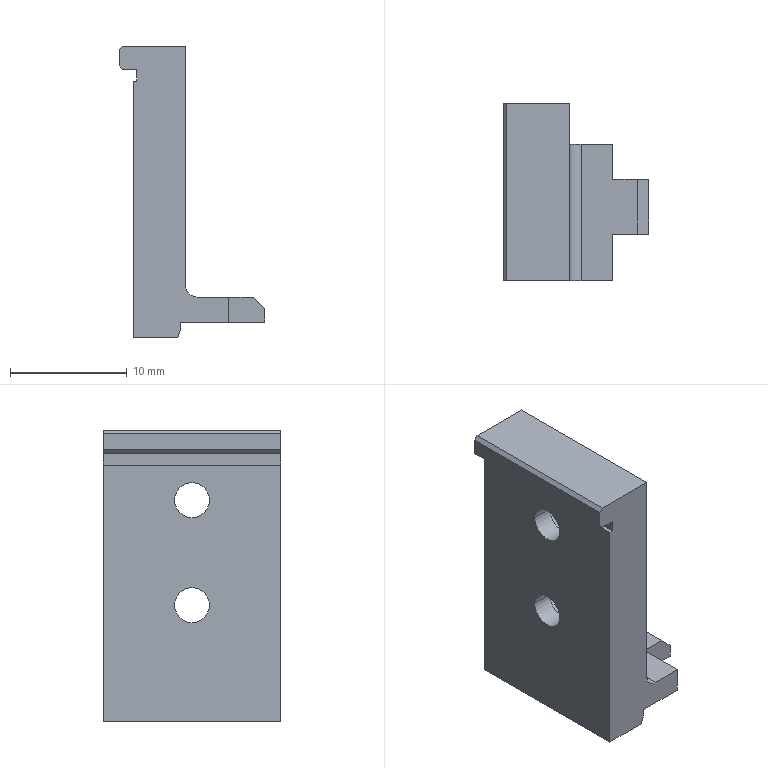Part | NX | 1 solid | 34 faces | box 12.5 x 15.2 x 25 mm | volume 1724 mm3 | plane 25 | cylinder 9 | commonest cylinder face diameters 3 x4 5 x4 2 x1
STEP:
#1=CARTESIAN_POINT('',(-1.77,0.,-1.43));
#2=VERTEX_POINT('',#1);
#3=CARTESIAN_POINT('',(-2.025,0.,-2.13));
#4=VERTEX_POINT('',#3);
#5=CARTESIAN_POINT('',(-1.25,0.,0.));
#6=DIRECTION('',(-0.342,0.,-0.9397));
#7=VECTOR('',#6,1000.);
#8=LINE('',#5,#7);
#9=EDGE_CURVE('',#2,#4,#8,.T.);
#10=ORIENTED_EDGE('',*,*,#9,.T.);
#11=CARTESIAN_POINT('',(-5.85,0.,-2.13));
#12=VERTEX_POINT('',#11);
#13=CARTESIAN_POINT('',(0.,0.,-2.13));
#14=DIRECTION('',(1.,0.,0.));
#15=VECTOR('',#14,1000.);
#16=LINE('',#13,#15);
#17=EDGE_CURVE('',#12,#4,#16,.T.);
#18=ORIENTED_EDGE('',*,*,#17,.F.);
#19=CARTESIAN_POINT('',(-5.85,0.,19.87));
#20=VERTEX_POINT('',#19);
#21=CARTESIAN_POINT('',(-5.85,0.,0.));
#22=DIRECTION('',(0.,0.,1.));
#23=VECTOR('',#22,1000.);
#24=LINE('',#21,#23);
#25=EDGE_CURVE('',#12,#20,#24,.T.);
#26=ORIENTED_EDGE('',*,*,#25,.T.);
#27=CARTESIAN_POINT('',(-5.55,0.,19.87));
#28=VERTEX_POINT('',#27);
#29=CARTESIAN_POINT('',(0.,0.,19.87));
#30=DIRECTION('',(1.,0.,0.));
#31=VECTOR('',#30,1000.);
#32=LINE('',#29,#31);
#33=EDGE_CURVE('',#20,#28,#32,.T.);
#34=ORIENTED_EDGE('',*,*,#33,.T.);
#35=CARTESIAN_POINT('',(-5.55,0.,20.87));
#36=VERTEX_POINT('',#35);
#37=CARTESIAN_POINT('',(-5.55,0.,0.));
#38=DIRECTION('',(0.,0.,1.));
#39=VECTOR('',#38,1000.);
#40=LINE('',#37,#39);
#41=EDGE_CURVE('',#28,#36,#40,.T.);
#42=ORIENTED_EDGE('',*,*,#41,.T.);
#43=CARTESIAN_POINT('',(-6.75,0.,20.87));
#44=VERTEX_POINT('',#43);
#45=CARTESIAN_POINT('',(0.,0.,20.87));
#46=DIRECTION('',(-1.,0.,0.));
#47=VECTOR('',#46,1000.);
#48=LINE('',#45,#47);
#49=EDGE_CURVE('',#36,#44,#48,.T.);
#50=ORIENTED_EDGE('',*,*,#49,.T.);
#51=CARTESIAN_POINT('',(-7.05,0.,21.17));
#52=VERTEX_POINT('',#51);
#53=CARTESIAN_POINT('',(14.12,0.,0.));
#54=DIRECTION('',(0.7071,0.,-0.7071));
#55=VECTOR('',#54,1000.);
#56=LINE('',#53,#55);
#57=EDGE_CURVE('',#52,#44,#56,.T.);
#58=ORIENTED_EDGE('',*,*,#57,.F.);
#59=CARTESIAN_POINT('',(-7.05,0.,22.57));
#60=VERTEX_POINT('',#59);
#61=CARTESIAN_POINT('',(-7.05,0.,0.));
#62=DIRECTION('',(0.,0.,1.));
#63=VECTOR('',#62,1000.);
#64=LINE('',#61,#63);
#65=EDGE_CURVE('',#52,#60,#64,.T.);
#66=ORIENTED_EDGE('',*,*,#65,.T.);
#67=CARTESIAN_POINT('',(-6.75,0.,22.87));
#68=VERTEX_POINT('',#67);
#69=CARTESIAN_POINT('',(-29.62,0.,0.));
#70=DIRECTION('',(0.7071,0.,0.7071));
#71=VECTOR('',#70,1000.);
#72=LINE('',#69,#71);
#73=EDGE_CURVE('',#60,#68,#72,.T.);
#74=ORIENTED_EDGE('',*,*,#73,.T.);
#75=CARTESIAN_POINT('',(-1.35,0.,22.87));
#76=VERTEX_POINT('',#75);
#77=CARTESIAN_POINT('',(0.,0.,22.87));
#78=DIRECTION('',(1.,0.,0.));
#79=VECTOR('',#78,1000.);
#80=LINE('',#77,#79);
#81=EDGE_CURVE('',#68,#76,#80,.T.);
#82=ORIENTED_EDGE('',*,*,#81,.T.);
#83=CARTESIAN_POINT('',(-1.35,0.,-0.78));
#84=VERTEX_POINT('',#83);
#85=CARTESIAN_POINT('',(-1.35,0.,0.));
#86=DIRECTION('',(0.,0.,1.));
#87=VECTOR('',#86,1000.);
#88=LINE('',#85,#87);
#89=EDGE_CURVE('',#84,#76,#88,.T.);
#90=ORIENTED_EDGE('',*,*,#89,.F.);
#91=CARTESIAN_POINT('',(-1.77,0.,-0.78));
#92=VERTEX_POINT('',#91);
#93=CARTESIAN_POINT('',(0.,0.,-0.78));
#94=DIRECTION('',(-1.,0.,0.));
#95=VECTOR('',#94,1000.);
#96=LINE('',#93,#95);
#97=EDGE_CURVE('',#84,#92,#96,.T.);
#98=ORIENTED_EDGE('',*,*,#97,.T.);
#99=CARTESIAN_POINT('',(-1.77,0.,0.));
#100=DIRECTION('',(0.,0.,-1.));
#101=VECTOR('',#100,1000.);
#102=LINE('',#99,#101);
#103=EDGE_CURVE('',#92,#2,#102,.T.);
#104=ORIENTED_EDGE('',*,*,#103,.T.);
#105=EDGE_LOOP('',(#10,#18,#26,#34,#42,#50,#58,#66,#74,#82,#90,#98,#104));
#106=FACE_BOUND('',#105,.T.);
#107=CARTESIAN_POINT('',(0.,0.,0.));
#108=DIRECTION('',(0.,-1.,0.));
#109=DIRECTION('',(0.,0.,-1.));
#110=AXIS2_PLACEMENT_3D('',#107,#108,#109);
#111=PLANE('',#110);
#112=ADVANCED_FACE('',(#106),#111,.F.);
#113=CARTESIAN_POINT('',(-1.77,-15.2,-1.43));
#114=VERTEX_POINT('',#113);
#115=CARTESIAN_POINT('',(-1.77,0.,-1.43));
#116=DIRECTION('',(0.,-1.,0.));
#117=VECTOR('',#116,1000.);
#118=LINE('',#115,#117);
#119=EDGE_CURVE('',#2,#114,#118,.T.);
#120=ORIENTED_EDGE('',*,*,#119,.F.);
#121=ORIENTED_EDGE('',*,*,#103,.F.);
#122=CARTESIAN_POINT('',(-1.77,-15.2,-0.78));
#123=VERTEX_POINT('',#122);
#124=CARTESIAN_POINT('',(-1.77,0.,-0.78));
#125=DIRECTION('',(0.,-1.,0.));
#126=VECTOR('',#125,1000.);
#127=LINE('',#124,#126);
#128=EDGE_CURVE('',#92,#123,#127,.T.);
#129=ORIENTED_EDGE('',*,*,#128,.T.);
#130=CARTESIAN_POINT('',(-1.77,-15.2,0.));
#131=DIRECTION('',(0.,0.,1.));
#132=VECTOR('',#131,1000.);
#133=LINE('',#130,#132);
#134=EDGE_CURVE('',#114,#123,#133,.T.);
#135=ORIENTED_EDGE('',*,*,#134,.F.);
#136=EDGE_LOOP('',(#120,#121,#129,#135));
#137=FACE_BOUND('',#136,.T.);
#138=CARTESIAN_POINT('',(-1.77,0.,-0.93));
#139=DIRECTION('',(1.,0.,0.));
#140=DIRECTION('',(0.,1.,0.));
#141=AXIS2_PLACEMENT_3D('',#138,#139,#140);
#142=PLANE('',#141);
#143=ADVANCED_FACE('',(#137),#142,.T.);
#144=CARTESIAN_POINT('',(-0.35,-15.2,1.37));
#145=VERTEX_POINT('',#144);
#146=CARTESIAN_POINT('',(2.35,-15.2,1.37));
#147=VERTEX_POINT('',#146);
#148=CARTESIAN_POINT('',(0.,-15.2,1.37));
#149=DIRECTION('',(1.,0.,0.));
#150=VECTOR('',#149,1000.);
#151=LINE('',#148,#150);
#152=EDGE_CURVE('',#145,#147,#151,.T.);
#153=ORIENTED_EDGE('',*,*,#152,.F.);
#154=CARTESIAN_POINT('',(-1.35,-15.2,2.37));
#155=VERTEX_POINT('',#154);
#156=CARTESIAN_POINT('',(-0.35,-15.2,2.37));
#157=DIRECTION('',(0.,1.,0.));
#158=DIRECTION('',(-1.,0.,0.));
#159=AXIS2_PLACEMENT_3D('',#156,#157,#158);
#160=CIRCLE('',#159,1.);
#161=EDGE_CURVE('',#145,#155,#160,.T.);
#162=ORIENTED_EDGE('',*,*,#161,.T.);
#163=CARTESIAN_POINT('',(-1.35,-15.2,22.87));
#164=VERTEX_POINT('',#163);
#165=CARTESIAN_POINT('',(-1.35,-15.2,0.));
#166=DIRECTION('',(0.,0.,-1.));
#167=VECTOR('',#166,1000.);
#168=LINE('',#165,#167);
#169=EDGE_CURVE('',#164,#155,#168,.T.);
#170=ORIENTED_EDGE('',*,*,#169,.F.);
#171=CARTESIAN_POINT('',(-6.75,-15.2,22.87));
#172=VERTEX_POINT('',#171);
#173=CARTESIAN_POINT('',(0.,-15.2,22.87));
#174=DIRECTION('',(-1.,0.,0.));
#175=VECTOR('',#174,1000.);
#176=LINE('',#173,#175);
#177=EDGE_CURVE('',#164,#172,#176,.T.);
#178=ORIENTED_EDGE('',*,*,#177,.T.);
#179=CARTESIAN_POINT('',(-7.05,-15.2,22.57));
#180=VERTEX_POINT('',#179);
#181=CARTESIAN_POINT('',(-29.62,-15.2,0.));
#182=DIRECTION('',(-0.7071,0.,-0.7071));
#183=VECTOR('',#182,1000.);
#184=LINE('',#181,#183);
#185=EDGE_CURVE('',#172,#180,#184,.T.);
#186=ORIENTED_EDGE('',*,*,#185,.T.);
#187=CARTESIAN_POINT('',(-7.05,-15.2,21.17));
#188=VERTEX_POINT('',#187);
#189=CARTESIAN_POINT('',(-7.05,-15.2,0.));
#190=DIRECTION('',(0.,0.,-1.));
#191=VECTOR('',#190,1000.);
#192=LINE('',#189,#191);
#193=EDGE_CURVE('',#180,#188,#192,.T.);
#194=ORIENTED_EDGE('',*,*,#193,.T.);
#195=CARTESIAN_POINT('',(-6.75,-15.2,20.87));
#196=VERTEX_POINT('',#195);
#197=CARTESIAN_POINT('',(14.12,-15.2,0.));
#198=DIRECTION('',(-0.7071,0.,0.7071));
#199=VECTOR('',#198,1000.);
#200=LINE('',#197,#199);
#201=EDGE_CURVE('',#196,#188,#200,.T.);
#202=ORIENTED_EDGE('',*,*,#201,.F.);
#203=CARTESIAN_POINT('',(-5.55,-15.2,20.87));
#204=VERTEX_POINT('',#203);
#205=CARTESIAN_POINT('',(0.,-15.2,20.87));
#206=DIRECTION('',(1.,0.,0.));
#207=VECTOR('',#206,1000.);
#208=LINE('',#205,#207);
#209=EDGE_CURVE('',#196,#204,#208,.T.);
#210=ORIENTED_EDGE('',*,*,#209,.T.);
#211=CARTESIAN_POINT('',(-5.55,-15.2,19.87));
#212=VERTEX_POINT('',#211);
#213=CARTESIAN_POINT('',(-5.55,-15.2,0.));
#214=DIRECTION('',(0.,0.,-1.));
#215=VECTOR('',#214,1000.);
#216=LINE('',#213,#215);
#217=EDGE_CURVE('',#204,#212,#216,.T.);
#218=ORIENTED_EDGE('',*,*,#217,.T.);
#219=CARTESIAN_POINT('',(-5.85,-15.2,19.87));
#220=VERTEX_POINT('',#219);
#221=CARTESIAN_POINT('',(0.,-15.2,19.87));
#222=DIRECTION('',(-1.,0.,0.));
#223=VECTOR('',#222,1000.);
#224=LINE('',#221,#223);
#225=EDGE_CURVE('',#212,#220,#224,.T.);
#226=ORIENTED_EDGE('',*,*,#225,.T.);
#227=CARTESIAN_POINT('',(-5.85,-15.2,-2.13));
#228=VERTEX_POINT('',#227);
#229=CARTESIAN_POINT('',(-5.85,-15.2,0.));
#230=DIRECTION('',(0.,0.,-1.));
#231=VECTOR('',#230,1000.);
#232=LINE('',#229,#231);
#233=EDGE_CURVE('',#220,#228,#232,.T.);
#234=ORIENTED_EDGE('',*,*,#233,.T.);
#235=CARTESIAN_POINT('',(-2.025,-15.2,-2.13));
#236=VERTEX_POINT('',#235);
#237=CARTESIAN_POINT('',(0.,-15.2,-2.13));
#238=DIRECTION('',(-1.,0.,0.));
#239=VECTOR('',#238,1000.);
#240=LINE('',#237,#239);
#241=EDGE_CURVE('',#236,#228,#240,.T.);
#242=ORIENTED_EDGE('',*,*,#241,.F.);
#243=CARTESIAN_POINT('',(-1.25,-15.2,0.));
#244=DIRECTION('',(0.342,0.,0.9397));
#245=VECTOR('',#244,1000.);
#246=LINE('',#243,#245);
#247=EDGE_CURVE('',#236,#114,#246,.T.);
#248=ORIENTED_EDGE('',*,*,#247,.T.);
#249=ORIENTED_EDGE('',*,*,#134,.T.);
#250=CARTESIAN_POINT('',(2.35,-15.2,-0.78));
#251=VERTEX_POINT('',#250);
#252=CARTESIAN_POINT('',(0.,-15.2,-0.78));
#253=DIRECTION('',(1.,0.,0.));
#254=VECTOR('',#253,1000.);
#255=LINE('',#252,#254);
#256=EDGE_CURVE('',#123,#251,#255,.T.);
#257=ORIENTED_EDGE('',*,*,#256,.T.);
#258=CARTESIAN_POINT('',(2.35,-15.2,0.));
#259=DIRECTION('',(0.,0.,-1.));
#260=VECTOR('',#259,1000.);
#261=LINE('',#258,#260);
#262=EDGE_CURVE('',#147,#251,#261,.T.);
#263=ORIENTED_EDGE('',*,*,#262,.F.);
#264=EDGE_LOOP('',(#153,#162,#170,#178,#186,#194,#202,#210,#218,#226,#234,#242,#248,#249,#257,#263));
#265=FACE_BOUND('',#264,.T.);
#266=CARTESIAN_POINT('',(-1.35,-15.2,0.));
#267=DIRECTION('',(0.,1.,0.));
#268=DIRECTION('',(1.,0.,0.));
#269=AXIS2_PLACEMENT_3D('',#266,#267,#268);
#270=PLANE('',#269);
#271=ADVANCED_FACE('',(#265),#270,.F.);
#272=CARTESIAN_POINT('',(-4.05,-5.1,7.87));
#273=VERTEX_POINT('',#272);
#274=CARTESIAN_POINT('',(-4.05,-10.1,7.87));
#275=VERTEX_POINT('',#274);
#276=CARTESIAN_POINT('',(-4.05,-7.6,7.87));
#277=DIRECTION('',(1.,0.,0.));
#278=DIRECTION('',(0.,-1.,0.));
#279=AXIS2_PLACEMENT_3D('',#276,#277,#278);
#280=CIRCLE('',#279,2.5);
#281=EDGE_CURVE('',#273,#275,#280,.T.);
#282=ORIENTED_EDGE('',*,*,#281,.T.);
#283=CARTESIAN_POINT('',(-4.05,-7.6,7.87));
#284=DIRECTION('',(1.,0.,0.));
#285=DIRECTION('',(0.,-1.,0.));
#286=AXIS2_PLACEMENT_3D('',#283,#284,#285);
#287=CIRCLE('',#286,2.5);
#288=EDGE_CURVE('',#275,#273,#287,.T.);
#289=ORIENTED_EDGE('',*,*,#288,.T.);
#290=EDGE_LOOP('',(#282,#289));
#291=FACE_BOUND('',#290,.T.);
#292=CARTESIAN_POINT('',(-4.05,-6.1,7.87));
#293=VERTEX_POINT('',#292);
#294=CARTESIAN_POINT('',(-4.05,-9.1,7.87));
#295=VERTEX_POINT('',#294);
#296=CARTESIAN_POINT('',(-4.05,-7.6,7.87));
#297=DIRECTION('',(1.,0.,0.));
#298=DIRECTION('',(0.,-1.,0.));
#299=AXIS2_PLACEMENT_3D('',#296,#297,#298);
#300=CIRCLE('',#299,1.5);
#301=EDGE_CURVE('',#293,#295,#300,.T.);
#302=ORIENTED_EDGE('',*,*,#301,.F.);
#303=CARTESIAN_POINT('',(-4.05,-7.6,7.87));
#304=DIRECTION('',(1.,0.,0.));
#305=DIRECTION('',(0.,-1.,0.));
#306=AXIS2_PLACEMENT_3D('',#303,#304,#305);
#307=CIRCLE('',#306,1.5);
#308=EDGE_CURVE('',#295,#293,#307,.T.);
#309=ORIENTED_EDGE('',*,*,#308,.F.);
#310=EDGE_LOOP('',(#302,#309));
#311=FACE_BOUND('',#310,.T.);
#312=CARTESIAN_POINT('',(-4.05,-7.6,7.87));
#313=DIRECTION('',(-1.,0.,0.));
#314=DIRECTION('',(0.,0.,1.));
#315=AXIS2_PLACEMENT_3D('',#312,#313,#314);
#316=PLANE('',#315);
#317=ADVANCED_FACE('',(#291,#311),#316,.F.);
#318=ORIENTED_EDGE('',*,*,#241,.T.);
#319=CARTESIAN_POINT('',(-5.85,0.,-2.13));
#320=DIRECTION('',(0.,1.,0.));
#321=VECTOR('',#320,1000.);
#322=LINE('',#319,#321);
#323=EDGE_CURVE('',#228,#12,#322,.T.);
#324=ORIENTED_EDGE('',*,*,#323,.T.);
#325=ORIENTED_EDGE('',*,*,#17,.T.);
#326=CARTESIAN_POINT('',(-2.025,0.,-2.13));
#327=DIRECTION('',(0.,-1.,0.));
#328=VECTOR('',#327,1000.);
#329=LINE('',#326,#328);
#330=EDGE_CURVE('',#4,#236,#329,.T.);
#331=ORIENTED_EDGE('',*,*,#330,.T.);
#332=EDGE_LOOP('',(#318,#324,#325,#331));
#333=FACE_BOUND('',#332,.T.);
#334=CARTESIAN_POINT('',(0.,0.,-2.13));
#335=DIRECTION('',(0.,0.,1.));
#336=DIRECTION('',(1.,0.,0.));
#337=AXIS2_PLACEMENT_3D('',#334,#335,#336);
#338=PLANE('',#337);
#339=ADVANCED_FACE('',(#333),#338,.F.);
#340=ORIENTED_EDGE('',*,*,#9,.F.);
#341=ORIENTED_EDGE('',*,*,#119,.T.);
#342=ORIENTED_EDGE('',*,*,#247,.F.);
#343=ORIENTED_EDGE('',*,*,#330,.F.);
#344=EDGE_LOOP('',(#340,#341,#342,#343));
#345=FACE_BOUND('',#344,.T.);
#346=CARTESIAN_POINT('',(-2.025,-15.2,-2.13));
#347=DIRECTION('',(0.9397,0.,-0.342));
#348=DIRECTION('',(0.,-1.,0.));
#349=AXIS2_PLACEMENT_3D('',#346,#347,#348);
#350=PLANE('',#349);
#351=ADVANCED_FACE('',(#345),#350,.T.);
#352=CARTESIAN_POINT('',(-5.85,0.,19.87));
#353=DIRECTION('',(0.,-1.,0.));
#354=VECTOR('',#353,1000.);
#355=LINE('',#352,#354);
#356=EDGE_CURVE('',#20,#220,#355,.T.);
#357=ORIENTED_EDGE('',*,*,#356,.T.);
#358=ORIENTED_EDGE('',*,*,#225,.F.);
#359=CARTESIAN_POINT('',(-5.55,0.,19.87));
#360=DIRECTION('',(0.,-1.,0.));
#361=VECTOR('',#360,1000.);
#362=LINE('',#359,#361);
#363=EDGE_CURVE('',#28,#212,#362,.T.);
#364=ORIENTED_EDGE('',*,*,#363,.F.);
#365=ORIENTED_EDGE('',*,*,#33,.F.);
#366=EDGE_LOOP('',(#357,#358,#364,#365));
#367=FACE_BOUND('',#366,.T.);
#368=CARTESIAN_POINT('',(-4.85,0.,19.87));
#369=DIRECTION('',(0.,0.,1.));
#370=DIRECTION('',(1.,0.,0.));
#371=AXIS2_PLACEMENT_3D('',#368,#369,#370);
#372=PLANE('',#371);
#373=ADVANCED_FACE('',(#367),#372,.T.);
#374=ORIENTED_EDGE('',*,*,#363,.T.);
#375=ORIENTED_EDGE('',*,*,#217,.F.);
#376=CARTESIAN_POINT('',(-5.55,0.,20.87));
#377=DIRECTION('',(0.,-1.,0.));
#378=VECTOR('',#377,1000.);
#379=LINE('',#376,#378);
#380=EDGE_CURVE('',#36,#204,#379,.T.);
#381=ORIENTED_EDGE('',*,*,#380,.F.);
#382=ORIENTED_EDGE('',*,*,#41,.F.);
#383=EDGE_LOOP('',(#374,#375,#381,#382));
#384=FACE_BOUND('',#383,.T.);
#385=CARTESIAN_POINT('',(-5.55,0.,19.87));
#386=DIRECTION('',(-1.,0.,0.));
#387=DIRECTION('',(0.,0.,1.));
#388=AXIS2_PLACEMENT_3D('',#385,#386,#387);
#389=PLANE('',#388);
#390=ADVANCED_FACE('',(#384),#389,.T.);
#391=CARTESIAN_POINT('',(-6.75,0.,20.87));
#392=DIRECTION('',(0.,1.,0.));
#393=VECTOR('',#392,1000.);
#394=LINE('',#391,#393);
#395=EDGE_CURVE('',#196,#44,#394,.T.);
#396=ORIENTED_EDGE('',*,*,#395,.T.);
#397=ORIENTED_EDGE('',*,*,#49,.F.);
#398=ORIENTED_EDGE('',*,*,#380,.T.);
#399=ORIENTED_EDGE('',*,*,#209,.F.);
#400=EDGE_LOOP('',(#396,#397,#398,#399));
#401=FACE_BOUND('',#400,.T.);
#402=CARTESIAN_POINT('',(-4.85,0.,20.87));
#403=DIRECTION('',(0.,0.,-1.));
#404=DIRECTION('',(0.,-1.,0.));
#405=AXIS2_PLACEMENT_3D('',#402,#403,#404);
#406=PLANE('',#405);
#407=ADVANCED_FACE('',(#401),#406,.T.);
#408=CARTESIAN_POINT('',(-7.05,0.,22.57));
#409=DIRECTION('',(0.,-1.,0.));
#410=VECTOR('',#409,1000.);
#411=LINE('',#408,#410);
#412=EDGE_CURVE('',#60,#180,#411,.T.);
#413=ORIENTED_EDGE('',*,*,#412,.F.);
#414=ORIENTED_EDGE('',*,*,#65,.F.);
#415=CARTESIAN_POINT('',(-7.05,0.,21.17));
#416=DIRECTION('',(0.,-1.,0.));
#417=VECTOR('',#416,1000.);
#418=LINE('',#415,#417);
#419=EDGE_CURVE('',#52,#188,#418,.T.);
#420=ORIENTED_EDGE('',*,*,#419,.T.);
#421=ORIENTED_EDGE('',*,*,#193,.F.);
#422=EDGE_LOOP('',(#413,#414,#420,#421));
#423=FACE_BOUND('',#422,.T.);
#424=CARTESIAN_POINT('',(-7.05,0.,20.87));
#425=DIRECTION('',(-1.,0.,0.));
#426=DIRECTION('',(0.,0.,1.));
#427=AXIS2_PLACEMENT_3D('',#424,#425,#426);
#428=PLANE('',#427);
#429=ADVANCED_FACE('',(#423),#428,.T.);
#430=CARTESIAN_POINT('',(-6.75,0.,22.87));
#431=DIRECTION('',(0.,1.,0.));
#432=VECTOR('',#431,1000.);
#433=LINE('',#430,#432);
#434=EDGE_CURVE('',#172,#68,#433,.T.);
#435=ORIENTED_EDGE('',*,*,#434,.F.);
#436=ORIENTED_EDGE('',*,*,#177,.F.);
#437=CARTESIAN_POINT('',(-1.35,0.,22.87));
#438=DIRECTION('',(0.,-1.,0.));
#439=VECTOR('',#438,1000.);
#440=LINE('',#437,#439);
#441=EDGE_CURVE('',#76,#164,#440,.T.);
#442=ORIENTED_EDGE('',*,*,#441,.F.);
#443=ORIENTED_EDGE('',*,*,#81,.F.);
#444=EDGE_LOOP('',(#435,#436,#442,#443));
#445=FACE_BOUND('',#444,.T.);
#446=CARTESIAN_POINT('',(-6.05,0.,22.87));
#447=DIRECTION('',(0.,0.,1.));
#448=DIRECTION('',(1.,0.,0.));
#449=AXIS2_PLACEMENT_3D('',#446,#447,#448);
#450=PLANE('',#449);
#451=ADVANCED_FACE('',(#445),#450,.T.);
#452=ORIENTED_EDGE('',*,*,#323,.F.);
#453=ORIENTED_EDGE('',*,*,#233,.F.);
#454=ORIENTED_EDGE('',*,*,#356,.F.);
#455=ORIENTED_EDGE('',*,*,#25,.F.);
#456=EDGE_LOOP('',(#452,#453,#454,#455));
#457=FACE_BOUND('',#456,.T.);
#458=CARTESIAN_POINT('',(-5.85,-6.1,16.87));
#459=VERTEX_POINT('',#458);
#460=CARTESIAN_POINT('',(-5.85,-9.1,16.87));
#461=VERTEX_POINT('',#460);
#462=CARTESIAN_POINT('',(-5.85,-7.6,16.87));
#463=DIRECTION('',(1.,0.,0.));
#464=DIRECTION('',(0.,-1.,0.));
#465=AXIS2_PLACEMENT_3D('',#462,#463,#464);
#466=CIRCLE('',#465,1.5);
#467=EDGE_CURVE('',#459,#461,#466,.T.);
#468=ORIENTED_EDGE('',*,*,#467,.T.);
#469=CARTESIAN_POINT('',(-5.85,-7.6,16.87));
#470=DIRECTION('',(1.,0.,0.));
#471=DIRECTION('',(0.,-1.,0.));
#472=AXIS2_PLACEMENT_3D('',#469,#470,#471);
#473=CIRCLE('',#472,1.5);
#474=EDGE_CURVE('',#461,#459,#473,.T.);
#475=ORIENTED_EDGE('',*,*,#474,.T.);
#476=EDGE_LOOP('',(#468,#475));
#477=FACE_BOUND('',#476,.T.);
#478=CARTESIAN_POINT('',(-5.85,-9.1,7.87));
#479=VERTEX_POINT('',#478);
#480=CARTESIAN_POINT('',(-5.85,-6.1,7.87));
#481=VERTEX_POINT('',#480);
#482=CARTESIAN_POINT('',(-5.85,-7.6,7.87));
#483=DIRECTION('',(1.,0.,0.));
#484=DIRECTION('',(0.,-1.,0.));
#485=AXIS2_PLACEMENT_3D('',#482,#483,#484);
#486=CIRCLE('',#485,1.5);
#487=EDGE_CURVE('',#479,#481,#486,.T.);
#488=ORIENTED_EDGE('',*,*,#487,.T.);
#489=CARTESIAN_POINT('',(-5.85,-7.6,7.87));
#490=DIRECTION('',(1.,0.,0.));
#491=DIRECTION('',(0.,-1.,0.));
#492=AXIS2_PLACEMENT_3D('',#489,#490,#491);
#493=CIRCLE('',#492,1.5);
#494=EDGE_CURVE('',#481,#479,#493,.T.);
#495=ORIENTED_EDGE('',*,*,#494,.T.);
#496=EDGE_LOOP('',(#488,#495));
#497=FACE_BOUND('',#496,.T.);
#498=CARTESIAN_POINT('',(-5.85,0.,-1.13));
#499=DIRECTION('',(-1.,0.,0.));
#500=DIRECTION('',(0.,0.,1.));
#501=AXIS2_PLACEMENT_3D('',#498,#499,#500);
#502=PLANE('',#501);
#503=ADVANCED_FACE('',(#457,#477,#497),#502,.T.);
#504=CARTESIAN_POINT('',(-1.35,-3.5,2.37));
#505=VERTEX_POINT('',#504);
#506=CARTESIAN_POINT('',(-1.35,-15.285,2.37));
#507=DIRECTION('',(0.,1.,0.));
#508=VECTOR('',#507,1000.);
#509=LINE('',#506,#508);
#510=EDGE_CURVE('',#155,#505,#509,.T.);
#511=ORIENTED_EDGE('',*,*,#510,.F.);
#512=ORIENTED_EDGE('',*,*,#161,.F.);
#513=CARTESIAN_POINT('',(-0.35,-3.5,1.37));
#514=VERTEX_POINT('',#513);
#515=CARTESIAN_POINT('',(-0.35,-15.2,1.37));
#516=DIRECTION('',(0.,1.,0.));
#517=VECTOR('',#516,1000.);
#518=LINE('',#515,#517);
#519=EDGE_CURVE('',#145,#514,#518,.T.);
#520=ORIENTED_EDGE('',*,*,#519,.T.);
#521=CARTESIAN_POINT('',(-0.35,-3.5,2.37));
#522=DIRECTION('',(0.,1.,0.));
#523=DIRECTION('',(-1.,0.,0.));
#524=AXIS2_PLACEMENT_3D('',#521,#522,#523);
#525=CIRCLE('',#524,1.);
#526=EDGE_CURVE('',#514,#505,#525,.T.);
#527=ORIENTED_EDGE('',*,*,#526,.T.);
#528=EDGE_LOOP('',(#511,#512,#520,#527));
#529=FACE_BOUND('',#528,.T.);
#530=CARTESIAN_POINT('',(-0.35,-15.285,2.37));
#531=DIRECTION('',(0.,1.,0.));
#532=DIRECTION('',(-1.,0.,0.));
#533=AXIS2_PLACEMENT_3D('',#530,#531,#532);
#534=CYLINDRICAL_SURFACE('',#533,1.);
#535=ADVANCED_FACE('',(#529),#534,.F.);
#536=CARTESIAN_POINT('',(2.35,-3.5,-0.78));
#537=VERTEX_POINT('',#536);
#538=CARTESIAN_POINT('',(2.35,-3.5,1.37));
#539=VERTEX_POINT('',#538);
#540=CARTESIAN_POINT('',(2.35,-3.5,0.));
#541=DIRECTION('',(0.,0.,1.));
#542=VECTOR('',#541,1000.);
#543=LINE('',#540,#542);
#544=EDGE_CURVE('',#537,#539,#543,.T.);
#545=ORIENTED_EDGE('',*,*,#544,.F.);
#546=CARTESIAN_POINT('',(-1.35,-3.5,-0.78));
#547=VERTEX_POINT('',#546);
#548=CARTESIAN_POINT('',(0.,-3.5,-0.78));
#549=DIRECTION('',(1.,0.,0.));
#550=VECTOR('',#549,1000.);
#551=LINE('',#548,#550);
#552=EDGE_CURVE('',#547,#537,#551,.T.);
#553=ORIENTED_EDGE('',*,*,#552,.F.);
#554=CARTESIAN_POINT('',(-1.35,-3.5,0.));
#555=DIRECTION('',(0.,0.,1.));
#556=VECTOR('',#555,1000.);
#557=LINE('',#554,#556);
#558=EDGE_CURVE('',#547,#505,#557,.T.);
#559=ORIENTED_EDGE('',*,*,#558,.T.);
#560=ORIENTED_EDGE('',*,*,#526,.F.);
#561=CARTESIAN_POINT('',(0.,-3.5,1.37));
#562=DIRECTION('',(1.,0.,0.));
#563=VECTOR('',#562,1000.);
#564=LINE('',#561,#563);
#565=EDGE_CURVE('',#514,#539,#564,.T.);
#566=ORIENTED_EDGE('',*,*,#565,.T.);
#567=EDGE_LOOP('',(#545,#553,#559,#560,#566));
#568=FACE_BOUND('',#567,.T.);
#569=CARTESIAN_POINT('',(-1.77,-3.5,-0.83));
#570=DIRECTION('',(0.,-1.,0.));
#571=DIRECTION('',(0.,0.,-1.));
#572=AXIS2_PLACEMENT_3D('',#569,#570,#571);
#573=PLANE('',#572);
#574=ADVANCED_FACE('',(#568),#573,.F.);
#575=ORIENTED_EDGE('',*,*,#262,.T.);
#576=CARTESIAN_POINT('',(2.35,-11.2,-0.78));
#577=VERTEX_POINT('',#576);
#578=CARTESIAN_POINT('',(2.35,0.,-0.78));
#579=DIRECTION('',(0.,-1.,0.));
#580=VECTOR('',#579,1000.);
#581=LINE('',#578,#580);
#582=EDGE_CURVE('',#577,#251,#581,.T.);
#583=ORIENTED_EDGE('',*,*,#582,.F.);
#584=CARTESIAN_POINT('',(2.35,-11.2,1.37));
#585=VERTEX_POINT('',#584);
#586=CARTESIAN_POINT('',(2.35,-11.2,0.));
#587=DIRECTION('',(0.,0.,1.));
#588=VECTOR('',#587,1000.);
#589=LINE('',#586,#588);
#590=EDGE_CURVE('',#577,#585,#589,.T.);
#591=ORIENTED_EDGE('',*,*,#590,.T.);
#592=CARTESIAN_POINT('',(2.35,0.,1.37));
#593=DIRECTION('',(0.,-1.,0.));
#594=VECTOR('',#593,1000.);
#595=LINE('',#592,#594);
#596=EDGE_CURVE('',#585,#147,#595,.T.);
#597=ORIENTED_EDGE('',*,*,#596,.T.);
#598=EDGE_LOOP('',(#575,#583,#591,#597));
#599=FACE_BOUND('',#598,.T.);
#600=CARTESIAN_POINT('',(2.35,0.,52.77));
#601=DIRECTION('',(-1.,0.,0.));
#602=DIRECTION('',(0.,0.,1.));
#603=AXIS2_PLACEMENT_3D('',#600,#601,#602);
#604=PLANE('',#603);
#605=ADVANCED_FACE('',(#599),#604,.F.);
#606=ORIENTED_EDGE('',*,*,#281,.F.);
#607=CARTESIAN_POINT('',(-1.35,-5.1,7.87));
#608=VERTEX_POINT('',#607);
#609=CARTESIAN_POINT('',(-7.072,-5.1,7.87));
#610=DIRECTION('',(1.,0.,0.));
#611=VECTOR('',#610,1000.);
#612=LINE('',#609,#611);
#613=EDGE_CURVE('',#608,#273,#612,.F.);
#614=ORIENTED_EDGE('',*,*,#613,.F.);
#615=CARTESIAN_POINT('',(-1.35,-10.1,7.87));
#616=VERTEX_POINT('',#615);
#617=CARTESIAN_POINT('',(-1.35,-7.6,7.87));
#618=DIRECTION('',(1.,0.,0.));
#619=DIRECTION('',(0.,-1.,0.));
#620=AXIS2_PLACEMENT_3D('',#617,#618,#619);
#621=CIRCLE('',#620,2.5);
#622=EDGE_CURVE('',#608,#616,#621,.T.);
#623=ORIENTED_EDGE('',*,*,#622,.T.);
#624=CARTESIAN_POINT('',(-7.072,-10.1,7.87));
#625=DIRECTION('',(1.,0.,0.));
#626=VECTOR('',#625,1000.);
#627=LINE('',#624,#626);
#628=EDGE_CURVE('',#616,#275,#627,.F.);
#629=ORIENTED_EDGE('',*,*,#628,.T.);
#630=EDGE_LOOP('',(#606,#614,#623,#629));
#631=FACE_BOUND('',#630,.T.);
#632=CARTESIAN_POINT('',(-7.072,-7.6,7.87));
#633=DIRECTION('',(1.,0.,0.));
#634=DIRECTION('',(0.,-1.,0.));
#635=AXIS2_PLACEMENT_3D('',#632,#633,#634);
#636=CYLINDRICAL_SURFACE('',#635,2.5);
#637=ADVANCED_FACE('',(#631),#636,.F.);
#638=ORIENTED_EDGE('',*,*,#565,.F.);
#639=ORIENTED_EDGE('',*,*,#519,.F.);
#640=ORIENTED_EDGE('',*,*,#152,.T.);
#641=ORIENTED_EDGE('',*,*,#596,.F.);
#642=CARTESIAN_POINT('',(4.45,-11.2,1.37));
#643=VERTEX_POINT('',#642);
#644=CARTESIAN_POINT('',(0.,-11.2,1.37));
#645=DIRECTION('',(-1.,0.,0.));
#646=VECTOR('',#645,1000.);
#647=LINE('',#644,#646);
#648=EDGE_CURVE('',#643,#585,#647,.T.);
#649=ORIENTED_EDGE('',*,*,#648,.F.);
#650=CARTESIAN_POINT('',(4.45,-6.5,1.37));
#651=VERTEX_POINT('',#650);
#652=CARTESIAN_POINT('',(4.45,0.,1.37));
#653=DIRECTION('',(0.,-1.,0.));
#654=VECTOR('',#653,1000.);
#655=LINE('',#652,#654);
#656=EDGE_CURVE('',#651,#643,#655,.T.);
#657=ORIENTED_EDGE('',*,*,#656,.F.);
#658=CARTESIAN_POINT('',(2.35,-6.5,1.37));
#659=VERTEX_POINT('',#658);
#660=CARTESIAN_POINT('',(0.,-6.5,1.37));
#661=DIRECTION('',(1.,0.,0.));
#662=VECTOR('',#661,1000.);
#663=LINE('',#660,#662);
#664=EDGE_CURVE('',#659,#651,#663,.T.);
#665=ORIENTED_EDGE('',*,*,#664,.F.);
#666=CARTESIAN_POINT('',(2.35,0.,1.37));
#667=DIRECTION('',(0.,-1.,0.));
#668=VECTOR('',#667,1000.);
#669=LINE('',#666,#668);
#670=EDGE_CURVE('',#539,#659,#669,.T.);
#671=ORIENTED_EDGE('',*,*,#670,.F.);
#672=EDGE_LOOP('',(#638,#639,#640,#641,#649,#657,#665,#671));
#673=FACE_BOUND('',#672,.T.);
#674=CARTESIAN_POINT('',(-1.35,-15.2,1.37));
#675=DIRECTION('',(0.,0.,-1.));
#676=DIRECTION('',(0.,-1.,0.));
#677=AXIS2_PLACEMENT_3D('',#674,#675,#676);
#678=PLANE('',#677);
#679=ADVANCED_FACE('',(#673),#678,.F.);
#680=ORIENTED_EDGE('',*,*,#590,.F.);
#681=CARTESIAN_POINT('',(5.45,-11.2,-0.78));
#682=VERTEX_POINT('',#681);
#683=CARTESIAN_POINT('',(0.,-11.2,-0.78));
#684=DIRECTION('',(1.,0.,0.));
#685=VECTOR('',#684,1000.);
#686=LINE('',#683,#685);
#687=EDGE_CURVE('',#577,#682,#686,.T.);
#688=ORIENTED_EDGE('',*,*,#687,.T.);
#689=CARTESIAN_POINT('',(5.45,-11.2,0.37));
#690=VERTEX_POINT('',#689);
#691=CARTESIAN_POINT('',(5.45,-11.2,0.));
#692=DIRECTION('',(0.,0.,-1.));
#693=VECTOR('',#692,1000.);
#694=LINE('',#691,#693);
#695=EDGE_CURVE('',#690,#682,#694,.T.);
#696=ORIENTED_EDGE('',*,*,#695,.F.);
#697=CARTESIAN_POINT('',(5.82,-11.2,0.));
#698=DIRECTION('',(-0.7071,0.,0.7071));
#699=VECTOR('',#698,1000.);
#700=LINE('',#697,#699);
#701=EDGE_CURVE('',#690,#643,#700,.T.);
#702=ORIENTED_EDGE('',*,*,#701,.T.);
#703=ORIENTED_EDGE('',*,*,#648,.T.);
#704=EDGE_LOOP('',(#680,#688,#696,#702,#703));
#705=FACE_BOUND('',#704,.T.);
#706=CARTESIAN_POINT('',(2.35,-11.2,-0.78));
#707=DIRECTION('',(0.,-1.,0.));
#708=DIRECTION('',(0.,0.,-1.));
#709=AXIS2_PLACEMENT_3D('',#706,#707,#708);
#710=PLANE('',#709);
#711=ADVANCED_FACE('',(#705),#710,.T.);
#712=CARTESIAN_POINT('',(5.45,-6.5,0.37));
#713=VERTEX_POINT('',#712);
#714=CARTESIAN_POINT('',(5.45,0.,0.37));
#715=DIRECTION('',(0.,-1.,0.));
#716=VECTOR('',#715,1000.);
#717=LINE('',#714,#716);
#718=EDGE_CURVE('',#713,#690,#717,.T.);
#719=ORIENTED_EDGE('',*,*,#718,.F.);
#720=CARTESIAN_POINT('',(5.82,-6.5,0.));
#721=DIRECTION('',(0.7071,0.,-0.7071));
#722=VECTOR('',#721,1000.);
#723=LINE('',#720,#722);
#724=EDGE_CURVE('',#651,#713,#723,.T.);
#725=ORIENTED_EDGE('',*,*,#724,.F.);
#726=ORIENTED_EDGE('',*,*,#656,.T.);
#727=ORIENTED_EDGE('',*,*,#701,.F.);
#728=EDGE_LOOP('',(#719,#725,#726,#727));
#729=FACE_BOUND('',#728,.T.);
#730=CARTESIAN_POINT('',(4.95,-8.85,0.87));
#731=DIRECTION('',(-0.7071,0.,-0.7071));
#732=DIRECTION('',(-0.7071,0.,0.7071));
#733=AXIS2_PLACEMENT_3D('',#730,#731,#732);
#734=PLANE('',#733);
#735=ADVANCED_FACE('',(#729),#734,.F.);
#736=ORIENTED_EDGE('',*,*,#718,.T.);
#737=ORIENTED_EDGE('',*,*,#695,.T.);
#738=CARTESIAN_POINT('',(5.45,-6.5,-0.78));
#739=VERTEX_POINT('',#738);
#740=CARTESIAN_POINT('',(5.45,0.,-0.78));
#741=DIRECTION('',(0.,1.,0.));
#742=VECTOR('',#741,1000.);
#743=LINE('',#740,#742);
#744=EDGE_CURVE('',#682,#739,#743,.T.);
#745=ORIENTED_EDGE('',*,*,#744,.T.);
#746=CARTESIAN_POINT('',(5.45,-6.5,0.));
#747=DIRECTION('',(0.,0.,1.));
#748=VECTOR('',#747,1000.);
#749=LINE('',#746,#748);
#750=EDGE_CURVE('',#739,#713,#749,.T.);
#751=ORIENTED_EDGE('',*,*,#750,.T.);
#752=EDGE_LOOP('',(#736,#737,#745,#751));
#753=FACE_BOUND('',#752,.T.);
#754=CARTESIAN_POINT('',(5.45,-10.254,0.812));
#755=DIRECTION('',(1.,0.,0.));
#756=DIRECTION('',(0.,1.,0.));
#757=AXIS2_PLACEMENT_3D('',#754,#755,#756);
#758=PLANE('',#757);
#759=ADVANCED_FACE('',(#753),#758,.T.);
#760=CARTESIAN_POINT('',(-1.35,-10.1,16.87));
#761=VERTEX_POINT('',#760);
#762=CARTESIAN_POINT('',(-1.35,-5.1,16.87));
#763=VERTEX_POINT('',#762);
#764=CARTESIAN_POINT('',(-1.35,-7.6,16.87));
#765=DIRECTION('',(1.,0.,0.));
#766=DIRECTION('',(0.,-1.,0.));
#767=AXIS2_PLACEMENT_3D('',#764,#765,#766);
#768=CIRCLE('',#767,2.5);
#769=EDGE_CURVE('',#761,#763,#768,.T.);
#770=ORIENTED_EDGE('',*,*,#769,.T.);
#771=CARTESIAN_POINT('',(-4.05,-5.1,16.87));
#772=VERTEX_POINT('',#771);
#773=CARTESIAN_POINT('',(-7.072,-5.1,16.87));
#774=DIRECTION('',(1.,0.,0.));
#775=VECTOR('',#774,1000.);
#776=LINE('',#773,#775);
#777=EDGE_CURVE('',#763,#772,#776,.F.);
#778=ORIENTED_EDGE('',*,*,#777,.T.);
#779=CARTESIAN_POINT('',(-4.05,-10.1,16.87));
#780=VERTEX_POINT('',#779);
#781=CARTESIAN_POINT('',(-4.05,-7.6,16.87));
#782=DIRECTION('',(1.,0.,0.));
#783=DIRECTION('',(0.,-1.,0.));
#784=AXIS2_PLACEMENT_3D('',#781,#782,#783);
#785=CIRCLE('',#784,2.5);
#786=EDGE_CURVE('',#780,#772,#785,.T.);
#787=ORIENTED_EDGE('',*,*,#786,.F.);
#788=CARTESIAN_POINT('',(-7.072,-10.1,16.87));
#789=DIRECTION('',(1.,0.,0.));
#790=VECTOR('',#789,1000.);
#791=LINE('',#788,#790);
#792=EDGE_CURVE('',#761,#780,#791,.F.);
#793=ORIENTED_EDGE('',*,*,#792,.F.);
#794=EDGE_LOOP('',(#770,#778,#787,#793));
#795=FACE_BOUND('',#794,.T.);
#796=CARTESIAN_POINT('',(-7.072,-7.6,16.87));
#797=DIRECTION('',(1.,0.,0.));
#798=DIRECTION('',(0.,-1.,0.));
#799=AXIS2_PLACEMENT_3D('',#796,#797,#798);
#800=CYLINDRICAL_SURFACE('',#799,2.5);
#801=ADVANCED_FACE('',(#795),#800,.F.);
#802=ORIENTED_EDGE('',*,*,#169,.T.);
#803=ORIENTED_EDGE('',*,*,#510,.T.);
#804=ORIENTED_EDGE('',*,*,#558,.F.);
#805=CARTESIAN_POINT('',(-1.35,0.,-0.78));
#806=DIRECTION('',(0.,-1.,0.));
#807=VECTOR('',#806,1000.);
#808=LINE('',#805,#807);
#809=EDGE_CURVE('',#84,#547,#808,.T.);
#810=ORIENTED_EDGE('',*,*,#809,.F.);
#811=ORIENTED_EDGE('',*,*,#89,.T.);
#812=ORIENTED_EDGE('',*,*,#441,.T.);
#813=EDGE_LOOP('',(#802,#803,#804,#810,#811,#812));
#814=FACE_BOUND('',#813,.T.);
#815=ORIENTED_EDGE('',*,*,#769,.F.);
#816=CARTESIAN_POINT('',(-1.35,-7.6,16.87));
#817=DIRECTION('',(1.,0.,0.));
#818=DIRECTION('',(0.,-1.,0.));
#819=AXIS2_PLACEMENT_3D('',#816,#817,#818);
#820=CIRCLE('',#819,2.5);
#821=EDGE_CURVE('',#763,#761,#820,.T.);
#822=ORIENTED_EDGE('',*,*,#821,.F.);
#823=EDGE_LOOP('',(#815,#822));
#824=FACE_BOUND('',#823,.T.);
#825=ORIENTED_EDGE('',*,*,#622,.F.);
#826=CARTESIAN_POINT('',(-1.35,-7.6,7.87));
#827=DIRECTION('',(1.,0.,0.));
#828=DIRECTION('',(0.,-1.,0.));
#829=AXIS2_PLACEMENT_3D('',#826,#827,#828);
#830=CIRCLE('',#829,2.5);
#831=EDGE_CURVE('',#616,#608,#830,.T.);
#832=ORIENTED_EDGE('',*,*,#831,.F.);
#833=EDGE_LOOP('',(#825,#832));
#834=FACE_BOUND('',#833,.T.);
#835=CARTESIAN_POINT('',(-1.35,0.,-1.13));
#836=DIRECTION('',(-1.,0.,0.));
#837=DIRECTION('',(0.,0.,1.));
#838=AXIS2_PLACEMENT_3D('',#835,#836,#837);
#839=PLANE('',#838);
#840=ADVANCED_FACE('',(#814,#824,#834),#839,.F.);
#841=ORIENTED_EDGE('',*,*,#786,.T.);
#842=CARTESIAN_POINT('',(-4.05,-7.6,16.87));
#843=DIRECTION('',(1.,0.,0.));
#844=DIRECTION('',(0.,-1.,0.));
#845=AXIS2_PLACEMENT_3D('',#842,#843,#844);
#846=CIRCLE('',#845,2.5);
#847=EDGE_CURVE('',#772,#780,#846,.T.);
#848=ORIENTED_EDGE('',*,*,#847,.T.);
#849=EDGE_LOOP('',(#841,#848));
#850=FACE_BOUND('',#849,.T.);
#851=CARTESIAN_POINT('',(-4.05,-9.1,16.87));
#852=VERTEX_POINT('',#851);
#853=CARTESIAN_POINT('',(-4.05,-6.1,16.87));
#854=VERTEX_POINT('',#853);
#855=CARTESIAN_POINT('',(-4.05,-7.6,16.87));
#856=DIRECTION('',(1.,0.,0.));
#857=DIRECTION('',(0.,-1.,0.));
#858=AXIS2_PLACEMENT_3D('',#855,#856,#857);
#859=CIRCLE('',#858,1.5);
#860=EDGE_CURVE('',#852,#854,#859,.T.);
#861=ORIENTED_EDGE('',*,*,#860,.F.);
#862=CARTESIAN_POINT('',(-4.05,-7.6,16.87));
#863=DIRECTION('',(1.,0.,0.));
#864=DIRECTION('',(0.,-1.,0.));
#865=AXIS2_PLACEMENT_3D('',#862,#863,#864);
#866=CIRCLE('',#865,1.5);
#867=EDGE_CURVE('',#854,#852,#866,.T.);
#868=ORIENTED_EDGE('',*,*,#867,.F.);
#869=EDGE_LOOP('',(#861,#868));
#870=FACE_BOUND('',#869,.T.);
#871=CARTESIAN_POINT('',(-4.05,-7.6,16.87));
#872=DIRECTION('',(-1.,0.,0.));
#873=DIRECTION('',(0.,0.,1.));
#874=AXIS2_PLACEMENT_3D('',#871,#872,#873);
#875=PLANE('',#874);
#876=ADVANCED_FACE('',(#850,#870),#875,.F.);
#877=ORIENTED_EDGE('',*,*,#467,.F.);
#878=CARTESIAN_POINT('',(-7.072,-6.1,16.87));
#879=DIRECTION('',(1.,0.,0.));
#880=VECTOR('',#879,1000.);
#881=LINE('',#878,#880);
#882=EDGE_CURVE('',#459,#854,#881,.T.);
#883=ORIENTED_EDGE('',*,*,#882,.T.);
#884=ORIENTED_EDGE('',*,*,#867,.T.);
#885=CARTESIAN_POINT('',(-7.072,-9.1,16.87));
#886=DIRECTION('',(1.,0.,0.));
#887=VECTOR('',#886,1000.);
#888=LINE('',#885,#887);
#889=EDGE_CURVE('',#461,#852,#888,.T.);
#890=ORIENTED_EDGE('',*,*,#889,.F.);
#891=EDGE_LOOP('',(#877,#883,#884,#890));
#892=FACE_BOUND('',#891,.T.);
#893=CARTESIAN_POINT('',(-7.072,-7.6,16.87));
#894=DIRECTION('',(1.,0.,0.));
#895=DIRECTION('',(0.,-1.,0.));
#896=AXIS2_PLACEMENT_3D('',#893,#894,#895);
#897=CYLINDRICAL_SURFACE('',#896,1.5);
#898=ADVANCED_FACE('',(#892),#897,.F.);
#899=ORIENTED_EDGE('',*,*,#301,.T.);
#900=CARTESIAN_POINT('',(-7.072,-9.1,7.87));
#901=DIRECTION('',(1.,0.,0.));
#902=VECTOR('',#901,1000.);
#903=LINE('',#900,#902);
#904=EDGE_CURVE('',#295,#479,#903,.F.);
#905=ORIENTED_EDGE('',*,*,#904,.T.);
#906=ORIENTED_EDGE('',*,*,#494,.F.);
#907=CARTESIAN_POINT('',(-7.072,-6.1,7.87));
#908=DIRECTION('',(1.,0.,0.));
#909=VECTOR('',#908,1000.);
#910=LINE('',#907,#909);
#911=EDGE_CURVE('',#293,#481,#910,.F.);
#912=ORIENTED_EDGE('',*,*,#911,.F.);
#913=EDGE_LOOP('',(#899,#905,#906,#912));
#914=FACE_BOUND('',#913,.T.);
#915=CARTESIAN_POINT('',(-7.072,-7.6,7.87));
#916=DIRECTION('',(1.,0.,0.));
#917=DIRECTION('',(0.,-1.,0.));
#918=AXIS2_PLACEMENT_3D('',#915,#916,#917);
#919=CYLINDRICAL_SURFACE('',#918,1.5);
#920=ADVANCED_FACE('',(#914),#919,.F.);
#921=ORIENTED_EDGE('',*,*,#412,.T.);
#922=ORIENTED_EDGE('',*,*,#185,.F.);
#923=ORIENTED_EDGE('',*,*,#434,.T.);
#924=ORIENTED_EDGE('',*,*,#73,.F.);
#925=EDGE_LOOP('',(#921,#922,#923,#924));
#926=FACE_BOUND('',#925,.T.);
#927=CARTESIAN_POINT('',(-6.9,-7.6,22.72));
#928=DIRECTION('',(-0.7071,0.,0.7071));
#929=DIRECTION('',(0.,1.,0.));
#930=AXIS2_PLACEMENT_3D('',#927,#928,#929);
#931=PLANE('',#930);
#932=ADVANCED_FACE('',(#926),#931,.T.);
#933=ORIENTED_EDGE('',*,*,#395,.F.);
#934=ORIENTED_EDGE('',*,*,#201,.T.);
#935=ORIENTED_EDGE('',*,*,#419,.F.);
#936=ORIENTED_EDGE('',*,*,#57,.T.);
#937=EDGE_LOOP('',(#933,#934,#935,#936));
#938=FACE_BOUND('',#937,.T.);
#939=CARTESIAN_POINT('',(-6.9,-7.6,21.02));
#940=DIRECTION('',(0.7071,0.,0.7071));
#941=DIRECTION('',(0.,-1.,0.));
#942=AXIS2_PLACEMENT_3D('',#939,#940,#941);
#943=PLANE('',#942);
#944=ADVANCED_FACE('',(#938),#943,.F.);
#945=CARTESIAN_POINT('',(2.35,-6.5,-0.78));
#946=VERTEX_POINT('',#945);
#947=CARTESIAN_POINT('',(2.35,-6.5,0.));
#948=DIRECTION('',(0.,0.,-1.));
#949=VECTOR('',#948,1000.);
#950=LINE('',#947,#949);
#951=EDGE_CURVE('',#659,#946,#950,.T.);
#952=ORIENTED_EDGE('',*,*,#951,.T.);
#953=CARTESIAN_POINT('',(2.35,0.,-0.78));
#954=DIRECTION('',(0.,-1.,0.));
#955=VECTOR('',#954,1000.);
#956=LINE('',#953,#955);
#957=EDGE_CURVE('',#537,#946,#956,.T.);
#958=ORIENTED_EDGE('',*,*,#957,.F.);
#959=ORIENTED_EDGE('',*,*,#544,.T.);
#960=ORIENTED_EDGE('',*,*,#670,.T.);
#961=EDGE_LOOP('',(#952,#958,#959,#960));
#962=FACE_BOUND('',#961,.T.);
#963=CARTESIAN_POINT('',(2.35,0.,52.77));
#964=DIRECTION('',(-1.,0.,0.));
#965=DIRECTION('',(0.,0.,1.));
#966=AXIS2_PLACEMENT_3D('',#963,#964,#965);
#967=PLANE('',#966);
#968=ADVANCED_FACE('',(#962),#967,.F.);
#969=CARTESIAN_POINT('',(0.,-6.5,-0.78));
#970=DIRECTION('',(1.,0.,0.));
#971=VECTOR('',#970,1000.);
#972=LINE('',#969,#971);
#973=EDGE_CURVE('',#946,#739,#972,.T.);
#974=ORIENTED_EDGE('',*,*,#973,.T.);
#975=ORIENTED_EDGE('',*,*,#744,.F.);
#976=ORIENTED_EDGE('',*,*,#687,.F.);
#977=ORIENTED_EDGE('',*,*,#582,.T.);
#978=ORIENTED_EDGE('',*,*,#256,.F.);
#979=ORIENTED_EDGE('',*,*,#128,.F.);
#980=ORIENTED_EDGE('',*,*,#97,.F.);
#981=ORIENTED_EDGE('',*,*,#809,.T.);
#982=ORIENTED_EDGE('',*,*,#552,.T.);
#983=ORIENTED_EDGE('',*,*,#957,.T.);
#984=EDGE_LOOP('',(#974,#975,#976,#977,#978,#979,#980,#981,#982,#983));
#985=FACE_BOUND('',#984,.T.);
#986=CARTESIAN_POINT('',(2.35,-6.5,-0.78));
#987=DIRECTION('',(0.,0.,-1.));
#988=DIRECTION('',(0.,-1.,0.));
#989=AXIS2_PLACEMENT_3D('',#986,#987,#988);
#990=PLANE('',#989);
#991=ADVANCED_FACE('',(#985),#990,.T.);
#992=ORIENTED_EDGE('',*,*,#951,.F.);
#993=ORIENTED_EDGE('',*,*,#664,.T.);
#994=ORIENTED_EDGE('',*,*,#724,.T.);
#995=ORIENTED_EDGE('',*,*,#750,.F.);
#996=ORIENTED_EDGE('',*,*,#973,.F.);
#997=EDGE_LOOP('',(#992,#993,#994,#995,#996));
#998=FACE_BOUND('',#997,.T.);
#999=CARTESIAN_POINT('',(2.35,-6.5,1.37));
#1000=DIRECTION('',(0.,1.,0.));
#1001=DIRECTION('',(1.,0.,0.));
#1002=AXIS2_PLACEMENT_3D('',#999,#1000,#1001);
#1003=PLANE('',#1002);
#1004=ADVANCED_FACE('',(#998),#1003,.T.);
#1005=ORIENTED_EDGE('',*,*,#628,.F.);
#1006=ORIENTED_EDGE('',*,*,#831,.T.);
#1007=ORIENTED_EDGE('',*,*,#613,.T.);
#1008=ORIENTED_EDGE('',*,*,#288,.F.);
#1009=EDGE_LOOP('',(#1005,#1006,#1007,#1008));
#1010=FACE_BOUND('',#1009,.T.);
#1011=CARTESIAN_POINT('',(-7.072,-7.6,7.87));
#1012=DIRECTION('',(1.,0.,0.));
#1013=DIRECTION('',(0.,-1.,0.));
#1014=AXIS2_PLACEMENT_3D('',#1011,#1012,#1013);
#1015=CYLINDRICAL_SURFACE('',#1014,2.5);
#1016=ADVANCED_FACE('',(#1010),#1015,.F.);
#1017=ORIENTED_EDGE('',*,*,#792,.T.);
#1018=ORIENTED_EDGE('',*,*,#847,.F.);
#1019=ORIENTED_EDGE('',*,*,#777,.F.);
#1020=ORIENTED_EDGE('',*,*,#821,.T.);
#1021=EDGE_LOOP('',(#1017,#1018,#1019,#1020));
#1022=FACE_BOUND('',#1021,.T.);
#1023=CARTESIAN_POINT('',(-7.072,-7.6,16.87));
#1024=DIRECTION('',(1.,0.,0.));
#1025=DIRECTION('',(0.,-1.,0.));
#1026=AXIS2_PLACEMENT_3D('',#1023,#1024,#1025);
#1027=CYLINDRICAL_SURFACE('',#1026,2.5);
#1028=ADVANCED_FACE('',(#1022),#1027,.F.);
#1029=ORIENTED_EDGE('',*,*,#860,.T.);
#1030=ORIENTED_EDGE('',*,*,#882,.F.);
#1031=ORIENTED_EDGE('',*,*,#474,.F.);
#1032=ORIENTED_EDGE('',*,*,#889,.T.);
#1033=EDGE_LOOP('',(#1029,#1030,#1031,#1032));
#1034=FACE_BOUND('',#1033,.T.);
#1035=CARTESIAN_POINT('',(-7.072,-7.6,16.87));
#1036=DIRECTION('',(1.,0.,0.));
#1037=DIRECTION('',(0.,-1.,0.));
#1038=AXIS2_PLACEMENT_3D('',#1035,#1036,#1037);
#1039=CYLINDRICAL_SURFACE('',#1038,1.5);
#1040=ADVANCED_FACE('',(#1034),#1039,.F.);
#1041=ORIENTED_EDGE('',*,*,#487,.F.);
#1042=ORIENTED_EDGE('',*,*,#904,.F.);
#1043=ORIENTED_EDGE('',*,*,#308,.T.);
#1044=ORIENTED_EDGE('',*,*,#911,.T.);
#1045=EDGE_LOOP('',(#1041,#1042,#1043,#1044));
#1046=FACE_BOUND('',#1045,.T.);
#1047=CARTESIAN_POINT('',(-7.072,-7.6,7.87));
#1048=DIRECTION('',(1.,0.,0.));
#1049=DIRECTION('',(0.,-1.,0.));
#1050=AXIS2_PLACEMENT_3D('',#1047,#1048,#1049);
#1051=CYLINDRICAL_SURFACE('',#1050,1.5);
#1052=ADVANCED_FACE('',(#1046),#1051,.F.);
#1053=CLOSED_SHELL('',(#112,#143,#271,#317,#339,#351,#373,#390,#407,#429,#451,#503,#535,#574,#605,#637,#679,#711,#735,#759,#801,#840,#876,#898,#920,#932,#944,#968,#991,#1004,#1016,#1028,#1040,#1052));
#1054=MANIFOLD_SOLID_BREP('',#1053);
#1055=(LENGTH_UNIT()NAMED_UNIT(*)SI_UNIT(.MILLI.,.METRE.));
#1056=UNCERTAINTY_MEASURE_WITH_UNIT(LENGTH_MEASURE(0.00001),#1055,'','');
#1057=(NAMED_UNIT(*)PLANE_ANGLE_UNIT()SI_UNIT($,.RADIAN.));
#1058=(NAMED_UNIT(*)SI_UNIT($,.STERADIAN.)SOLID_ANGLE_UNIT());
#1059=(GEOMETRIC_REPRESENTATION_CONTEXT(3)GLOBAL_UNCERTAINTY_ASSIGNED_CONTEXT((#1056))GLOBAL_UNIT_ASSIGNED_CONTEXT((#1055,#1057,#1058))REPRESENTATION_CONTEXT('',''));
#1060=ADVANCED_BREP_SHAPE_REPRESENTATION('',(#1054),#1059);